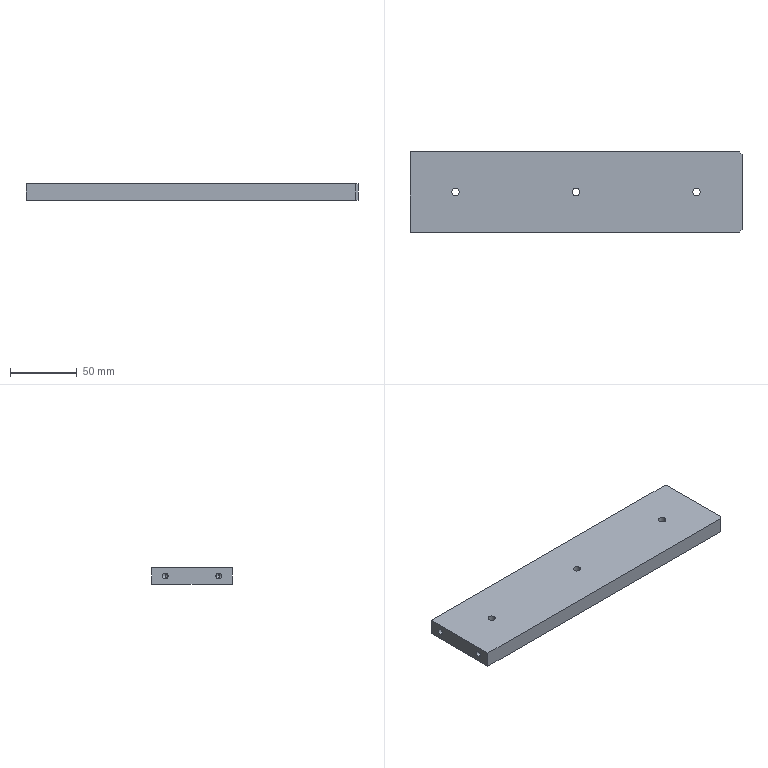Part | SolidWorks | features HoleWzd 2, Chamfer 1, Extrusion 1 | 1 solid | 31 faces | box 248 x 60 x 12 mm | volume 176365 mm3 | cylinder 16 | plane 11 | cone 4 | commonest cylinder face diameters 5.5 x6 10 x6 4.2 x4
STEP:
#1=CARTESIAN_POINT('',(95.,0.,-0.3));
#2=VERTEX_POINT('',#1);
#3=CARTESIAN_POINT('',(85.,0.,-0.3));
#4=VERTEX_POINT('',#3);
#5=CARTESIAN_POINT('',(90.,0.,-0.3));
#6=DIRECTION('',(0.,0.,-1.));
#7=DIRECTION('',(-1.,0.,0.));
#8=AXIS2_PLACEMENT_3D('',#5,#6,#7);
#9=CIRCLE('',#8,5.);
#10=EDGE_CURVE('',#2,#4,#9,.T.);
#11=ORIENTED_EDGE('',*,*,#10,.F.);
#12=CARTESIAN_POINT('',(95.,0.,-6.));
#13=VERTEX_POINT('',#12);
#14=CARTESIAN_POINT('',(95.,0.,-6.));
#15=DIRECTION('',(0.,0.,-1.));
#16=VECTOR('',#15,1000.);
#17=LINE('',#14,#16);
#18=EDGE_CURVE('',#2,#13,#17,.T.);
#19=ORIENTED_EDGE('',*,*,#18,.T.);
#20=CARTESIAN_POINT('',(85.,0.,-6.));
#21=VERTEX_POINT('',#20);
#22=CARTESIAN_POINT('',(90.,0.,-6.));
#23=DIRECTION('',(0.,0.,-1.));
#24=DIRECTION('',(-1.,0.,0.));
#25=AXIS2_PLACEMENT_3D('',#22,#23,#24);
#26=CIRCLE('',#25,5.);
#27=EDGE_CURVE('',#13,#21,#26,.T.);
#28=ORIENTED_EDGE('',*,*,#27,.T.);
#29=CARTESIAN_POINT('',(85.,0.,-6.));
#30=DIRECTION('',(0.,0.,-1.));
#31=VECTOR('',#30,1000.);
#32=LINE('',#29,#31);
#33=EDGE_CURVE('',#4,#21,#32,.T.);
#34=ORIENTED_EDGE('',*,*,#33,.F.);
#35=EDGE_LOOP('',(#11,#19,#28,#34));
#36=FACE_OUTER_BOUND('',#35,.T.);
#37=CARTESIAN_POINT('',(90.,0.,-6.));
#38=DIRECTION('',(0.,0.,-1.));
#39=DIRECTION('',(-1.,0.,0.));
#40=AXIS2_PLACEMENT_3D('',#37,#38,#39);
#41=CYLINDRICAL_SURFACE('',#40,5.);
#42=ADVANCED_FACE('',(#36),#41,.F.);
#43=CARTESIAN_POINT('',(92.75,0.,6.));
#44=VERTEX_POINT('',#43);
#45=CARTESIAN_POINT('',(87.25,0.,6.));
#46=VERTEX_POINT('',#45);
#47=CARTESIAN_POINT('',(90.,0.,6.));
#48=DIRECTION('',(0.,0.,-1.));
#49=DIRECTION('',(-1.,0.,0.));
#50=AXIS2_PLACEMENT_3D('',#47,#48,#49);
#51=CIRCLE('',#50,2.75);
#52=EDGE_CURVE('',#44,#46,#51,.T.);
#53=ORIENTED_EDGE('',*,*,#52,.F.);
#54=CARTESIAN_POINT('',(92.75,0.,-0.3));
#55=VERTEX_POINT('',#54);
#56=CARTESIAN_POINT('',(92.75,0.,-6.));
#57=DIRECTION('',(0.,0.,-1.));
#58=VECTOR('',#57,1000.);
#59=LINE('',#56,#58);
#60=EDGE_CURVE('',#44,#55,#59,.T.);
#61=ORIENTED_EDGE('',*,*,#60,.T.);
#62=CARTESIAN_POINT('',(87.25,0.,-0.3));
#63=VERTEX_POINT('',#62);
#64=CARTESIAN_POINT('',(90.,0.,-0.3));
#65=DIRECTION('',(0.,0.,-1.));
#66=DIRECTION('',(-1.,0.,0.));
#67=AXIS2_PLACEMENT_3D('',#64,#65,#66);
#68=CIRCLE('',#67,2.75);
#69=EDGE_CURVE('',#55,#63,#68,.T.);
#70=ORIENTED_EDGE('',*,*,#69,.T.);
#71=CARTESIAN_POINT('',(87.25,0.,-6.));
#72=DIRECTION('',(0.,0.,-1.));
#73=VECTOR('',#72,1000.);
#74=LINE('',#71,#73);
#75=EDGE_CURVE('',#46,#63,#74,.T.);
#76=ORIENTED_EDGE('',*,*,#75,.F.);
#77=EDGE_LOOP('',(#53,#61,#70,#76));
#78=FACE_OUTER_BOUND('',#77,.T.);
#79=CARTESIAN_POINT('',(90.,0.,-6.));
#80=DIRECTION('',(0.,0.,-1.));
#81=DIRECTION('',(-1.,0.,0.));
#82=AXIS2_PLACEMENT_3D('',#79,#80,#81);
#83=CYLINDRICAL_SURFACE('',#82,2.75);
#84=ADVANCED_FACE('',(#78),#83,.F.);
#85=CARTESIAN_POINT('',(5.,0.,-0.3));
#86=VERTEX_POINT('',#85);
#87=CARTESIAN_POINT('',(-5.,0.,-0.3));
#88=VERTEX_POINT('',#87);
#89=CARTESIAN_POINT('',(0.,0.,-0.3));
#90=DIRECTION('',(0.,0.,-1.));
#91=DIRECTION('',(-1.,0.,0.));
#92=AXIS2_PLACEMENT_3D('',#89,#90,#91);
#93=CIRCLE('',#92,5.);
#94=EDGE_CURVE('',#86,#88,#93,.T.);
#95=ORIENTED_EDGE('',*,*,#94,.F.);
#96=CARTESIAN_POINT('',(5.,0.,-6.));
#97=VERTEX_POINT('',#96);
#98=CARTESIAN_POINT('',(5.,0.,-6.));
#99=DIRECTION('',(0.,0.,-1.));
#100=VECTOR('',#99,1000.);
#101=LINE('',#98,#100);
#102=EDGE_CURVE('',#86,#97,#101,.T.);
#103=ORIENTED_EDGE('',*,*,#102,.T.);
#104=CARTESIAN_POINT('',(-5.,0.,-6.));
#105=VERTEX_POINT('',#104);
#106=CARTESIAN_POINT('',(0.,0.,-6.));
#107=DIRECTION('',(0.,0.,-1.));
#108=DIRECTION('',(-1.,0.,0.));
#109=AXIS2_PLACEMENT_3D('',#106,#107,#108);
#110=CIRCLE('',#109,5.);
#111=EDGE_CURVE('',#97,#105,#110,.T.);
#112=ORIENTED_EDGE('',*,*,#111,.T.);
#113=CARTESIAN_POINT('',(-5.,0.,-6.));
#114=DIRECTION('',(0.,0.,-1.));
#115=VECTOR('',#114,1000.);
#116=LINE('',#113,#115);
#117=EDGE_CURVE('',#88,#105,#116,.T.);
#118=ORIENTED_EDGE('',*,*,#117,.F.);
#119=EDGE_LOOP('',(#95,#103,#112,#118));
#120=FACE_OUTER_BOUND('',#119,.T.);
#121=CARTESIAN_POINT('',(0.,0.,-6.));
#122=DIRECTION('',(0.,0.,-1.));
#123=DIRECTION('',(-1.,0.,0.));
#124=AXIS2_PLACEMENT_3D('',#121,#122,#123);
#125=CYLINDRICAL_SURFACE('',#124,5.);
#126=ADVANCED_FACE('',(#120),#125,.F.);
#127=CARTESIAN_POINT('',(2.75,0.,6.));
#128=VERTEX_POINT('',#127);
#129=CARTESIAN_POINT('',(-2.75,0.,6.));
#130=VERTEX_POINT('',#129);
#131=CARTESIAN_POINT('',(0.,0.,6.));
#132=DIRECTION('',(0.,0.,-1.));
#133=DIRECTION('',(-1.,0.,0.));
#134=AXIS2_PLACEMENT_3D('',#131,#132,#133);
#135=CIRCLE('',#134,2.75);
#136=EDGE_CURVE('',#128,#130,#135,.T.);
#137=ORIENTED_EDGE('',*,*,#136,.F.);
#138=CARTESIAN_POINT('',(2.75,0.,-0.3));
#139=VERTEX_POINT('',#138);
#140=CARTESIAN_POINT('',(2.75,0.,-6.));
#141=DIRECTION('',(0.,0.,-1.));
#142=VECTOR('',#141,1000.);
#143=LINE('',#140,#142);
#144=EDGE_CURVE('',#128,#139,#143,.T.);
#145=ORIENTED_EDGE('',*,*,#144,.T.);
#146=CARTESIAN_POINT('',(-2.75,0.,-0.3));
#147=VERTEX_POINT('',#146);
#148=CARTESIAN_POINT('',(0.,0.,-0.3));
#149=DIRECTION('',(0.,0.,-1.));
#150=DIRECTION('',(-1.,0.,0.));
#151=AXIS2_PLACEMENT_3D('',#148,#149,#150);
#152=CIRCLE('',#151,2.75);
#153=EDGE_CURVE('',#139,#147,#152,.T.);
#154=ORIENTED_EDGE('',*,*,#153,.T.);
#155=CARTESIAN_POINT('',(-2.75,0.,-6.));
#156=DIRECTION('',(0.,0.,-1.));
#157=VECTOR('',#156,1000.);
#158=LINE('',#155,#157);
#159=EDGE_CURVE('',#130,#147,#158,.T.);
#160=ORIENTED_EDGE('',*,*,#159,.F.);
#161=EDGE_LOOP('',(#137,#145,#154,#160));
#162=FACE_OUTER_BOUND('',#161,.T.);
#163=CARTESIAN_POINT('',(0.,0.,-6.));
#164=DIRECTION('',(0.,0.,-1.));
#165=DIRECTION('',(-1.,0.,0.));
#166=AXIS2_PLACEMENT_3D('',#163,#164,#165);
#167=CYLINDRICAL_SURFACE('',#166,2.75);
#168=ADVANCED_FACE('',(#162),#167,.F.);
#169=CARTESIAN_POINT('',(-85.,0.,-0.3));
#170=VERTEX_POINT('',#169);
#171=CARTESIAN_POINT('',(-95.,0.,-0.3));
#172=VERTEX_POINT('',#171);
#173=CARTESIAN_POINT('',(-90.,0.,-0.3));
#174=DIRECTION('',(0.,0.,-1.));
#175=DIRECTION('',(-1.,0.,0.));
#176=AXIS2_PLACEMENT_3D('',#173,#174,#175);
#177=CIRCLE('',#176,5.);
#178=EDGE_CURVE('',#170,#172,#177,.T.);
#179=ORIENTED_EDGE('',*,*,#178,.F.);
#180=CARTESIAN_POINT('',(-85.,0.,-6.));
#181=VERTEX_POINT('',#180);
#182=CARTESIAN_POINT('',(-85.,0.,-6.));
#183=DIRECTION('',(0.,0.,-1.));
#184=VECTOR('',#183,1000.);
#185=LINE('',#182,#184);
#186=EDGE_CURVE('',#170,#181,#185,.T.);
#187=ORIENTED_EDGE('',*,*,#186,.T.);
#188=CARTESIAN_POINT('',(-95.,0.,-6.));
#189=VERTEX_POINT('',#188);
#190=CARTESIAN_POINT('',(-90.,0.,-6.));
#191=DIRECTION('',(0.,0.,-1.));
#192=DIRECTION('',(-1.,0.,0.));
#193=AXIS2_PLACEMENT_3D('',#190,#191,#192);
#194=CIRCLE('',#193,5.);
#195=EDGE_CURVE('',#181,#189,#194,.T.);
#196=ORIENTED_EDGE('',*,*,#195,.T.);
#197=CARTESIAN_POINT('',(-95.,0.,-6.));
#198=DIRECTION('',(0.,0.,-1.));
#199=VECTOR('',#198,1000.);
#200=LINE('',#197,#199);
#201=EDGE_CURVE('',#172,#189,#200,.T.);
#202=ORIENTED_EDGE('',*,*,#201,.F.);
#203=EDGE_LOOP('',(#179,#187,#196,#202));
#204=FACE_OUTER_BOUND('',#203,.T.);
#205=CARTESIAN_POINT('',(-90.,0.,-6.));
#206=DIRECTION('',(0.,0.,-1.));
#207=DIRECTION('',(-1.,0.,0.));
#208=AXIS2_PLACEMENT_3D('',#205,#206,#207);
#209=CYLINDRICAL_SURFACE('',#208,5.);
#210=ADVANCED_FACE('',(#204),#209,.F.);
#211=CARTESIAN_POINT('',(-87.25,0.,6.));
#212=VERTEX_POINT('',#211);
#213=CARTESIAN_POINT('',(-92.75,0.,6.));
#214=VERTEX_POINT('',#213);
#215=CARTESIAN_POINT('',(-90.,0.,6.));
#216=DIRECTION('',(0.,0.,-1.));
#217=DIRECTION('',(-1.,0.,0.));
#218=AXIS2_PLACEMENT_3D('',#215,#216,#217);
#219=CIRCLE('',#218,2.75);
#220=EDGE_CURVE('',#212,#214,#219,.T.);
#221=ORIENTED_EDGE('',*,*,#220,.F.);
#222=CARTESIAN_POINT('',(-87.25,0.,-0.3));
#223=VERTEX_POINT('',#222);
#224=CARTESIAN_POINT('',(-87.25,0.,-6.));
#225=DIRECTION('',(0.,0.,-1.));
#226=VECTOR('',#225,1000.);
#227=LINE('',#224,#226);
#228=EDGE_CURVE('',#212,#223,#227,.T.);
#229=ORIENTED_EDGE('',*,*,#228,.T.);
#230=CARTESIAN_POINT('',(-92.75,0.,-0.3));
#231=VERTEX_POINT('',#230);
#232=CARTESIAN_POINT('',(-90.,0.,-0.3));
#233=DIRECTION('',(0.,0.,-1.));
#234=DIRECTION('',(-1.,0.,0.));
#235=AXIS2_PLACEMENT_3D('',#232,#233,#234);
#236=CIRCLE('',#235,2.75);
#237=EDGE_CURVE('',#223,#231,#236,.T.);
#238=ORIENTED_EDGE('',*,*,#237,.T.);
#239=CARTESIAN_POINT('',(-92.75,0.,-6.));
#240=DIRECTION('',(0.,0.,-1.));
#241=VECTOR('',#240,1000.);
#242=LINE('',#239,#241);
#243=EDGE_CURVE('',#214,#231,#242,.T.);
#244=ORIENTED_EDGE('',*,*,#243,.F.);
#245=EDGE_LOOP('',(#221,#229,#238,#244));
#246=FACE_OUTER_BOUND('',#245,.T.);
#247=CARTESIAN_POINT('',(-90.,0.,-6.));
#248=DIRECTION('',(0.,0.,-1.));
#249=DIRECTION('',(-1.,0.,0.));
#250=AXIS2_PLACEMENT_3D('',#247,#248,#249);
#251=CYLINDRICAL_SURFACE('',#250,2.75);
#252=ADVANCED_FACE('',(#246),#251,.F.);
#253=CARTESIAN_POINT('',(-111.6,20.,-2.1));
#254=VERTEX_POINT('',#253);
#255=CARTESIAN_POINT('',(-111.6,20.,2.1));
#256=VERTEX_POINT('',#255);
#257=CARTESIAN_POINT('',(-111.6,20.,0.));
#258=DIRECTION('',(-1.,0.,0.));
#259=DIRECTION('',(0.,0.,1.));
#260=AXIS2_PLACEMENT_3D('',#257,#258,#259);
#261=CIRCLE('',#260,2.1);
#262=EDGE_CURVE('',#254,#256,#261,.T.);
#263=ORIENTED_EDGE('',*,*,#262,.F.);
#264=CARTESIAN_POINT('',(-124.,20.,-2.1));
#265=VERTEX_POINT('',#264);
#266=CARTESIAN_POINT('',(-124.,20.,-2.1));
#267=DIRECTION('',(-1.,0.,0.));
#268=VECTOR('',#267,1000.);
#269=LINE('',#266,#268);
#270=EDGE_CURVE('',#254,#265,#269,.T.);
#271=ORIENTED_EDGE('',*,*,#270,.T.);
#272=CARTESIAN_POINT('',(-124.,20.,2.1));
#273=VERTEX_POINT('',#272);
#274=CARTESIAN_POINT('',(-124.,20.,0.));
#275=DIRECTION('',(-1.,0.,0.));
#276=DIRECTION('',(0.,0.,1.));
#277=AXIS2_PLACEMENT_3D('',#274,#275,#276);
#278=CIRCLE('',#277,2.1);
#279=EDGE_CURVE('',#265,#273,#278,.T.);
#280=ORIENTED_EDGE('',*,*,#279,.T.);
#281=CARTESIAN_POINT('',(-124.,20.,2.1));
#282=DIRECTION('',(-1.,0.,0.));
#283=VECTOR('',#282,1000.);
#284=LINE('',#281,#283);
#285=EDGE_CURVE('',#256,#273,#284,.T.);
#286=ORIENTED_EDGE('',*,*,#285,.F.);
#287=EDGE_LOOP('',(#263,#271,#280,#286));
#288=FACE_OUTER_BOUND('',#287,.T.);
#289=CARTESIAN_POINT('',(-124.,20.,0.));
#290=DIRECTION('',(-1.,0.,0.));
#291=DIRECTION('',(0.,0.,1.));
#292=AXIS2_PLACEMENT_3D('',#289,#290,#291);
#293=CYLINDRICAL_SURFACE('',#292,2.1);
#294=ADVANCED_FACE('',(#288),#293,.F.);
#295=CARTESIAN_POINT('',(-110.338,20.,0.));
#296=VERTEX_POINT('',#295);
#297=CARTESIAN_POINT('',(-111.6,20.,2.1));
#298=DIRECTION('',(-0.515,0.,0.8572));
#299=VECTOR('',#298,1000.);
#300=LINE('',#297,#299);
#301=EDGE_CURVE('',#296,#256,#300,.T.);
#302=ORIENTED_EDGE('',*,*,#301,.F.);
#303=CARTESIAN_POINT('',(-111.6,20.,-2.1));
#304=DIRECTION('',(-0.515,0.,-0.8572));
#305=VECTOR('',#304,1000.);
#306=LINE('',#303,#305);
#307=EDGE_CURVE('',#296,#254,#306,.T.);
#308=ORIENTED_EDGE('',*,*,#307,.T.);
#309=ORIENTED_EDGE('',*,*,#262,.T.);
#310=EDGE_LOOP('',(#302,#308,#309));
#311=FACE_OUTER_BOUND('',#310,.T.);
#312=CARTESIAN_POINT('',(-111.6,20.,0.));
#313=DIRECTION('',(-1.,0.,0.));
#314=DIRECTION('',(0.,0.,1.));
#315=AXIS2_PLACEMENT_3D('',#312,#313,#314);
#316=CONICAL_SURFACE('',#315,2.1,1.03);
#317=ADVANCED_FACE('',(#311),#316,.F.);
#318=CARTESIAN_POINT('',(-111.6,-20.,-2.1));
#319=VERTEX_POINT('',#318);
#320=CARTESIAN_POINT('',(-111.6,-20.,2.1));
#321=VERTEX_POINT('',#320);
#322=CARTESIAN_POINT('',(-111.6,-20.,0.));
#323=DIRECTION('',(-1.,0.,0.));
#324=DIRECTION('',(0.,0.,1.));
#325=AXIS2_PLACEMENT_3D('',#322,#323,#324);
#326=CIRCLE('',#325,2.1);
#327=EDGE_CURVE('',#319,#321,#326,.T.);
#328=ORIENTED_EDGE('',*,*,#327,.F.);
#329=CARTESIAN_POINT('',(-124.,-20.,-2.1));
#330=VERTEX_POINT('',#329);
#331=CARTESIAN_POINT('',(-124.,-20.,-2.1));
#332=DIRECTION('',(-1.,0.,0.));
#333=VECTOR('',#332,1000.);
#334=LINE('',#331,#333);
#335=EDGE_CURVE('',#319,#330,#334,.T.);
#336=ORIENTED_EDGE('',*,*,#335,.T.);
#337=CARTESIAN_POINT('',(-124.,-20.,2.1));
#338=VERTEX_POINT('',#337);
#339=CARTESIAN_POINT('',(-124.,-20.,0.));
#340=DIRECTION('',(-1.,0.,0.));
#341=DIRECTION('',(0.,0.,1.));
#342=AXIS2_PLACEMENT_3D('',#339,#340,#341);
#343=CIRCLE('',#342,2.1);
#344=EDGE_CURVE('',#330,#338,#343,.T.);
#345=ORIENTED_EDGE('',*,*,#344,.T.);
#346=CARTESIAN_POINT('',(-124.,-20.,2.1));
#347=DIRECTION('',(-1.,0.,0.));
#348=VECTOR('',#347,1000.);
#349=LINE('',#346,#348);
#350=EDGE_CURVE('',#321,#338,#349,.T.);
#351=ORIENTED_EDGE('',*,*,#350,.F.);
#352=EDGE_LOOP('',(#328,#336,#345,#351));
#353=FACE_OUTER_BOUND('',#352,.T.);
#354=CARTESIAN_POINT('',(-124.,-20.,0.));
#355=DIRECTION('',(-1.,0.,0.));
#356=DIRECTION('',(0.,0.,1.));
#357=AXIS2_PLACEMENT_3D('',#354,#355,#356);
#358=CYLINDRICAL_SURFACE('',#357,2.1);
#359=ADVANCED_FACE('',(#353),#358,.F.);
#360=CARTESIAN_POINT('',(-110.338,-20.,0.));
#361=VERTEX_POINT('',#360);
#362=CARTESIAN_POINT('',(-111.6,-20.,2.1));
#363=DIRECTION('',(-0.515,0.,0.8572));
#364=VECTOR('',#363,1000.);
#365=LINE('',#362,#364);
#366=EDGE_CURVE('',#361,#321,#365,.T.);
#367=ORIENTED_EDGE('',*,*,#366,.F.);
#368=CARTESIAN_POINT('',(-111.6,-20.,-2.1));
#369=DIRECTION('',(-0.515,0.,-0.8572));
#370=VECTOR('',#369,1000.);
#371=LINE('',#368,#370);
#372=EDGE_CURVE('',#361,#319,#371,.T.);
#373=ORIENTED_EDGE('',*,*,#372,.T.);
#374=ORIENTED_EDGE('',*,*,#327,.T.);
#375=EDGE_LOOP('',(#367,#373,#374));
#376=FACE_OUTER_BOUND('',#375,.T.);
#377=CARTESIAN_POINT('',(-111.6,-20.,0.));
#378=DIRECTION('',(-1.,0.,0.));
#379=DIRECTION('',(0.,0.,1.));
#380=AXIS2_PLACEMENT_3D('',#377,#378,#379);
#381=CONICAL_SURFACE('',#380,2.1,1.03);
#382=ADVANCED_FACE('',(#376),#381,.F.);
#383=CARTESIAN_POINT('',(124.,-28.,6.));
#384=VERTEX_POINT('',#383);
#385=CARTESIAN_POINT('',(124.,28.,6.));
#386=VERTEX_POINT('',#385);
#387=CARTESIAN_POINT('',(124.,-30.,6.));
#388=DIRECTION('',(0.,1.,0.));
#389=VECTOR('',#388,1000.);
#390=LINE('',#387,#389);
#391=EDGE_CURVE('',#384,#386,#390,.T.);
#392=ORIENTED_EDGE('',*,*,#391,.F.);
#393=CARTESIAN_POINT('',(124.,-28.,-6.));
#394=VERTEX_POINT('',#393);
#395=CARTESIAN_POINT('',(124.,-28.,6.));
#396=DIRECTION('',(0.,0.,-1.));
#397=VECTOR('',#396,1000.);
#398=LINE('',#395,#397);
#399=EDGE_CURVE('',#384,#394,#398,.T.);
#400=ORIENTED_EDGE('',*,*,#399,.T.);
#401=CARTESIAN_POINT('',(124.,28.,-6.));
#402=VERTEX_POINT('',#401);
#403=CARTESIAN_POINT('',(124.,-30.,-6.));
#404=DIRECTION('',(0.,1.,0.));
#405=VECTOR('',#404,1000.);
#406=LINE('',#403,#405);
#407=EDGE_CURVE('',#394,#402,#406,.T.);
#408=ORIENTED_EDGE('',*,*,#407,.T.);
#409=CARTESIAN_POINT('',(124.,28.,6.));
#410=DIRECTION('',(0.,0.,1.));
#411=VECTOR('',#410,1000.);
#412=LINE('',#409,#411);
#413=EDGE_CURVE('',#402,#386,#412,.T.);
#414=ORIENTED_EDGE('',*,*,#413,.T.);
#415=EDGE_LOOP('',(#392,#400,#408,#414));
#416=FACE_OUTER_BOUND('',#415,.T.);
#417=CARTESIAN_POINT('',(124.,-30.,6.));
#418=DIRECTION('',(-1.,0.,0.));
#419=DIRECTION('',(0.,0.,1.));
#420=AXIS2_PLACEMENT_3D('',#417,#418,#419);
#421=PLANE('',#420);
#422=ADVANCED_FACE('',(#416),#421,.F.);
#423=CARTESIAN_POINT('',(122.,30.,6.));
#424=VERTEX_POINT('',#423);
#425=CARTESIAN_POINT('',(-124.,30.,6.));
#426=VERTEX_POINT('',#425);
#427=CARTESIAN_POINT('',(-124.,30.,6.));
#428=DIRECTION('',(-1.,0.,0.));
#429=VECTOR('',#428,1000.);
#430=LINE('',#427,#429);
#431=EDGE_CURVE('',#424,#426,#430,.T.);
#432=ORIENTED_EDGE('',*,*,#431,.F.);
#433=CARTESIAN_POINT('',(122.,30.,-6.));
#434=VERTEX_POINT('',#433);
#435=CARTESIAN_POINT('',(122.,30.,6.));
#436=DIRECTION('',(0.,0.,-1.));
#437=VECTOR('',#436,1000.);
#438=LINE('',#435,#437);
#439=EDGE_CURVE('',#424,#434,#438,.T.);
#440=ORIENTED_EDGE('',*,*,#439,.T.);
#441=CARTESIAN_POINT('',(-124.,30.,-6.));
#442=VERTEX_POINT('',#441);
#443=CARTESIAN_POINT('',(-124.,30.,-6.));
#444=DIRECTION('',(-1.,0.,0.));
#445=VECTOR('',#444,1000.);
#446=LINE('',#443,#445);
#447=EDGE_CURVE('',#434,#442,#446,.T.);
#448=ORIENTED_EDGE('',*,*,#447,.T.);
#449=CARTESIAN_POINT('',(-124.,30.,6.));
#450=DIRECTION('',(0.,0.,-1.));
#451=VECTOR('',#450,1000.);
#452=LINE('',#449,#451);
#453=EDGE_CURVE('',#426,#442,#452,.T.);
#454=ORIENTED_EDGE('',*,*,#453,.F.);
#455=EDGE_LOOP('',(#432,#440,#448,#454));
#456=FACE_OUTER_BOUND('',#455,.T.);
#457=CARTESIAN_POINT('',(-124.,30.,6.));
#458=DIRECTION('',(0.,-1.,0.));
#459=DIRECTION('',(0.,0.,-1.));
#460=AXIS2_PLACEMENT_3D('',#457,#458,#459);
#461=PLANE('',#460);
#462=ADVANCED_FACE('',(#456),#461,.F.);
#463=CARTESIAN_POINT('',(-124.,20.,0.));
#464=DIRECTION('',(-1.,0.,0.));
#465=DIRECTION('',(0.,0.,1.));
#466=AXIS2_PLACEMENT_3D('',#463,#464,#465);
#467=CIRCLE('',#466,2.1);
#468=EDGE_CURVE('',#273,#265,#467,.T.);
#469=ORIENTED_EDGE('',*,*,#468,.F.);
#470=ORIENTED_EDGE('',*,*,#279,.F.);
#471=EDGE_LOOP('',(#469,#470));
#472=FACE_BOUND('',#471,.T.);
#473=CARTESIAN_POINT('',(-124.,-20.,0.));
#474=DIRECTION('',(-1.,0.,0.));
#475=DIRECTION('',(0.,0.,1.));
#476=AXIS2_PLACEMENT_3D('',#473,#474,#475);
#477=CIRCLE('',#476,2.1);
#478=EDGE_CURVE('',#338,#330,#477,.T.);
#479=ORIENTED_EDGE('',*,*,#478,.F.);
#480=ORIENTED_EDGE('',*,*,#344,.F.);
#481=EDGE_LOOP('',(#479,#480));
#482=FACE_BOUND('',#481,.T.);
#483=CARTESIAN_POINT('',(-124.,-30.,-6.));
#484=VERTEX_POINT('',#483);
#485=CARTESIAN_POINT('',(-124.,-30.,-6.));
#486=DIRECTION('',(0.,-1.,0.));
#487=VECTOR('',#486,1000.);
#488=LINE('',#485,#487);
#489=EDGE_CURVE('',#442,#484,#488,.T.);
#490=ORIENTED_EDGE('',*,*,#489,.T.);
#491=CARTESIAN_POINT('',(-124.,-30.,6.));
#492=VERTEX_POINT('',#491);
#493=CARTESIAN_POINT('',(-124.,-30.,6.));
#494=DIRECTION('',(0.,0.,-1.));
#495=VECTOR('',#494,1000.);
#496=LINE('',#493,#495);
#497=EDGE_CURVE('',#492,#484,#496,.T.);
#498=ORIENTED_EDGE('',*,*,#497,.F.);
#499=CARTESIAN_POINT('',(-124.,-30.,6.));
#500=DIRECTION('',(0.,-1.,0.));
#501=VECTOR('',#500,1000.);
#502=LINE('',#499,#501);
#503=EDGE_CURVE('',#426,#492,#502,.T.);
#504=ORIENTED_EDGE('',*,*,#503,.F.);
#505=ORIENTED_EDGE('',*,*,#453,.T.);
#506=EDGE_LOOP('',(#490,#498,#504,#505));
#507=FACE_OUTER_BOUND('',#506,.T.);
#508=CARTESIAN_POINT('',(-124.,-30.,6.));
#509=DIRECTION('',(1.,0.,0.));
#510=DIRECTION('',(0.,0.,-1.));
#511=AXIS2_PLACEMENT_3D('',#508,#509,#510);
#512=PLANE('',#511);
#513=ADVANCED_FACE('',(#472,#482,#507),#512,.F.);
#514=CARTESIAN_POINT('',(122.,-30.,-6.));
#515=VERTEX_POINT('',#514);
#516=CARTESIAN_POINT('',(-124.,-30.,-6.));
#517=DIRECTION('',(1.,0.,0.));
#518=VECTOR('',#517,1000.);
#519=LINE('',#516,#518);
#520=EDGE_CURVE('',#484,#515,#519,.T.);
#521=ORIENTED_EDGE('',*,*,#520,.T.);
#522=CARTESIAN_POINT('',(122.,-30.,6.));
#523=VERTEX_POINT('',#522);
#524=CARTESIAN_POINT('',(122.,-30.,6.));
#525=DIRECTION('',(0.,0.,1.));
#526=VECTOR('',#525,1000.);
#527=LINE('',#524,#526);
#528=EDGE_CURVE('',#515,#523,#527,.T.);
#529=ORIENTED_EDGE('',*,*,#528,.T.);
#530=CARTESIAN_POINT('',(-124.,-30.,6.));
#531=DIRECTION('',(1.,0.,0.));
#532=VECTOR('',#531,1000.);
#533=LINE('',#530,#532);
#534=EDGE_CURVE('',#492,#523,#533,.T.);
#535=ORIENTED_EDGE('',*,*,#534,.F.);
#536=ORIENTED_EDGE('',*,*,#497,.T.);
#537=EDGE_LOOP('',(#521,#529,#535,#536));
#538=FACE_OUTER_BOUND('',#537,.T.);
#539=CARTESIAN_POINT('',(-124.,-30.,6.));
#540=DIRECTION('',(0.,1.,0.));
#541=DIRECTION('',(0.,0.,1.));
#542=AXIS2_PLACEMENT_3D('',#539,#540,#541);
#543=PLANE('',#542);
#544=ADVANCED_FACE('',(#538),#543,.F.);
#545=CARTESIAN_POINT('',(90.,0.,6.));
#546=DIRECTION('',(0.,0.,-1.));
#547=DIRECTION('',(-1.,0.,0.));
#548=AXIS2_PLACEMENT_3D('',#545,#546,#547);
#549=CIRCLE('',#548,2.75);
#550=EDGE_CURVE('',#46,#44,#549,.T.);
#551=ORIENTED_EDGE('',*,*,#550,.T.);
#552=ORIENTED_EDGE('',*,*,#52,.T.);
#553=EDGE_LOOP('',(#551,#552));
#554=FACE_BOUND('',#553,.T.);
#555=CARTESIAN_POINT('',(0.,0.,6.));
#556=DIRECTION('',(0.,0.,-1.));
#557=DIRECTION('',(-1.,0.,0.));
#558=AXIS2_PLACEMENT_3D('',#555,#556,#557);
#559=CIRCLE('',#558,2.75);
#560=EDGE_CURVE('',#130,#128,#559,.T.);
#561=ORIENTED_EDGE('',*,*,#560,.T.);
#562=ORIENTED_EDGE('',*,*,#136,.T.);
#563=EDGE_LOOP('',(#561,#562));
#564=FACE_BOUND('',#563,.T.);
#565=CARTESIAN_POINT('',(-90.,0.,6.));
#566=DIRECTION('',(0.,0.,-1.));
#567=DIRECTION('',(-1.,0.,0.));
#568=AXIS2_PLACEMENT_3D('',#565,#566,#567);
#569=CIRCLE('',#568,2.75);
#570=EDGE_CURVE('',#214,#212,#569,.T.);
#571=ORIENTED_EDGE('',*,*,#570,.T.);
#572=ORIENTED_EDGE('',*,*,#220,.T.);
#573=EDGE_LOOP('',(#571,#572));
#574=FACE_BOUND('',#573,.T.);
#575=ORIENTED_EDGE('',*,*,#534,.T.);
#576=CARTESIAN_POINT('',(124.,-28.,6.));
#577=DIRECTION('',(0.7071,0.7071,0.));
#578=VECTOR('',#577,1000.);
#579=LINE('',#576,#578);
#580=EDGE_CURVE('',#523,#384,#579,.T.);
#581=ORIENTED_EDGE('',*,*,#580,.T.);
#582=ORIENTED_EDGE('',*,*,#391,.T.);
#583=CARTESIAN_POINT('',(122.,30.,6.));
#584=DIRECTION('',(-0.7071,0.7071,0.));
#585=VECTOR('',#584,1000.);
#586=LINE('',#583,#585);
#587=EDGE_CURVE('',#386,#424,#586,.T.);
#588=ORIENTED_EDGE('',*,*,#587,.T.);
#589=ORIENTED_EDGE('',*,*,#431,.T.);
#590=ORIENTED_EDGE('',*,*,#503,.T.);
#591=EDGE_LOOP('',(#575,#581,#582,#588,#589,#590));
#592=FACE_OUTER_BOUND('',#591,.T.);
#593=CARTESIAN_POINT('',(0.,0.,6.));
#594=DIRECTION('',(0.,0.,-1.));
#595=DIRECTION('',(-1.,0.,0.));
#596=AXIS2_PLACEMENT_3D('',#593,#594,#595);
#597=PLANE('',#596);
#598=ADVANCED_FACE('',(#554,#564,#574,#592),#597,.F.);
#599=CARTESIAN_POINT('',(90.,0.,-6.));
#600=DIRECTION('',(0.,0.,-1.));
#601=DIRECTION('',(-1.,0.,0.));
#602=AXIS2_PLACEMENT_3D('',#599,#600,#601);
#603=CIRCLE('',#602,5.);
#604=EDGE_CURVE('',#21,#13,#603,.T.);
#605=ORIENTED_EDGE('',*,*,#604,.F.);
#606=ORIENTED_EDGE('',*,*,#27,.F.);
#607=EDGE_LOOP('',(#605,#606));
#608=FACE_BOUND('',#607,.T.);
#609=CARTESIAN_POINT('',(0.,0.,-6.));
#610=DIRECTION('',(0.,0.,-1.));
#611=DIRECTION('',(-1.,0.,0.));
#612=AXIS2_PLACEMENT_3D('',#609,#610,#611);
#613=CIRCLE('',#612,5.);
#614=EDGE_CURVE('',#105,#97,#613,.T.);
#615=ORIENTED_EDGE('',*,*,#614,.F.);
#616=ORIENTED_EDGE('',*,*,#111,.F.);
#617=EDGE_LOOP('',(#615,#616));
#618=FACE_BOUND('',#617,.T.);
#619=CARTESIAN_POINT('',(-90.,0.,-6.));
#620=DIRECTION('',(0.,0.,-1.));
#621=DIRECTION('',(-1.,0.,0.));
#622=AXIS2_PLACEMENT_3D('',#619,#620,#621);
#623=CIRCLE('',#622,5.);
#624=EDGE_CURVE('',#189,#181,#623,.T.);
#625=ORIENTED_EDGE('',*,*,#624,.F.);
#626=ORIENTED_EDGE('',*,*,#195,.F.);
#627=EDGE_LOOP('',(#625,#626));
#628=FACE_BOUND('',#627,.T.);
#629=ORIENTED_EDGE('',*,*,#407,.F.);
#630=CARTESIAN_POINT('',(76.,-76.,-6.));
#631=DIRECTION('',(-0.7071,-0.7071,0.));
#632=VECTOR('',#631,1000.);
#633=LINE('',#630,#632);
#634=EDGE_CURVE('',#394,#515,#633,.T.);
#635=ORIENTED_EDGE('',*,*,#634,.T.);
#636=ORIENTED_EDGE('',*,*,#520,.F.);
#637=ORIENTED_EDGE('',*,*,#489,.F.);
#638=ORIENTED_EDGE('',*,*,#447,.F.);
#639=CARTESIAN_POINT('',(76.,76.,-6.));
#640=DIRECTION('',(0.7071,-0.7071,0.));
#641=VECTOR('',#640,1000.);
#642=LINE('',#639,#641);
#643=EDGE_CURVE('',#434,#402,#642,.T.);
#644=ORIENTED_EDGE('',*,*,#643,.T.);
#645=EDGE_LOOP('',(#629,#635,#636,#637,#638,#644));
#646=FACE_OUTER_BOUND('',#645,.T.);
#647=CARTESIAN_POINT('',(0.,0.,-6.));
#648=DIRECTION('',(0.,0.,-1.));
#649=DIRECTION('',(-1.,0.,0.));
#650=AXIS2_PLACEMENT_3D('',#647,#648,#649);
#651=PLANE('',#650);
#652=ADVANCED_FACE('',(#608,#618,#628,#646),#651,.T.);
#653=ORIENTED_EDGE('',*,*,#372,.F.);
#654=ORIENTED_EDGE('',*,*,#366,.T.);
#655=CARTESIAN_POINT('',(-111.6,-20.,0.));
#656=DIRECTION('',(-1.,0.,0.));
#657=DIRECTION('',(0.,0.,1.));
#658=AXIS2_PLACEMENT_3D('',#655,#656,#657);
#659=CIRCLE('',#658,2.1);
#660=EDGE_CURVE('',#321,#319,#659,.T.);
#661=ORIENTED_EDGE('',*,*,#660,.T.);
#662=EDGE_LOOP('',(#653,#654,#661));
#663=FACE_OUTER_BOUND('',#662,.T.);
#664=CARTESIAN_POINT('',(-111.6,-20.,0.));
#665=DIRECTION('',(-1.,0.,0.));
#666=DIRECTION('',(0.,0.,1.));
#667=AXIS2_PLACEMENT_3D('',#664,#665,#666);
#668=CONICAL_SURFACE('',#667,2.1,1.03);
#669=ADVANCED_FACE('',(#663),#668,.F.);
#670=ORIENTED_EDGE('',*,*,#335,.F.);
#671=ORIENTED_EDGE('',*,*,#660,.F.);
#672=ORIENTED_EDGE('',*,*,#350,.T.);
#673=ORIENTED_EDGE('',*,*,#478,.T.);
#674=EDGE_LOOP('',(#670,#671,#672,#673));
#675=FACE_OUTER_BOUND('',#674,.T.);
#676=CARTESIAN_POINT('',(-124.,-20.,0.));
#677=DIRECTION('',(-1.,0.,0.));
#678=DIRECTION('',(0.,0.,1.));
#679=AXIS2_PLACEMENT_3D('',#676,#677,#678);
#680=CYLINDRICAL_SURFACE('',#679,2.1);
#681=ADVANCED_FACE('',(#675),#680,.F.);
#682=ORIENTED_EDGE('',*,*,#307,.F.);
#683=ORIENTED_EDGE('',*,*,#301,.T.);
#684=CARTESIAN_POINT('',(-111.6,20.,0.));
#685=DIRECTION('',(-1.,0.,0.));
#686=DIRECTION('',(0.,0.,1.));
#687=AXIS2_PLACEMENT_3D('',#684,#685,#686);
#688=CIRCLE('',#687,2.1);
#689=EDGE_CURVE('',#256,#254,#688,.T.);
#690=ORIENTED_EDGE('',*,*,#689,.T.);
#691=EDGE_LOOP('',(#682,#683,#690));
#692=FACE_OUTER_BOUND('',#691,.T.);
#693=CARTESIAN_POINT('',(-111.6,20.,0.));
#694=DIRECTION('',(-1.,0.,0.));
#695=DIRECTION('',(0.,0.,1.));
#696=AXIS2_PLACEMENT_3D('',#693,#694,#695);
#697=CONICAL_SURFACE('',#696,2.1,1.03);
#698=ADVANCED_FACE('',(#692),#697,.F.);
#699=ORIENTED_EDGE('',*,*,#270,.F.);
#700=ORIENTED_EDGE('',*,*,#689,.F.);
#701=ORIENTED_EDGE('',*,*,#285,.T.);
#702=ORIENTED_EDGE('',*,*,#468,.T.);
#703=EDGE_LOOP('',(#699,#700,#701,#702));
#704=FACE_OUTER_BOUND('',#703,.T.);
#705=CARTESIAN_POINT('',(-124.,20.,0.));
#706=DIRECTION('',(-1.,0.,0.));
#707=DIRECTION('',(0.,0.,1.));
#708=AXIS2_PLACEMENT_3D('',#705,#706,#707);
#709=CYLINDRICAL_SURFACE('',#708,2.1);
#710=ADVANCED_FACE('',(#704),#709,.F.);
#711=ORIENTED_EDGE('',*,*,#580,.F.);
#712=ORIENTED_EDGE('',*,*,#528,.F.);
#713=ORIENTED_EDGE('',*,*,#634,.F.);
#714=ORIENTED_EDGE('',*,*,#399,.F.);
#715=EDGE_LOOP('',(#711,#712,#713,#714));
#716=FACE_OUTER_BOUND('',#715,.T.);
#717=CARTESIAN_POINT('',(124.,-28.,6.));
#718=DIRECTION('',(-0.7071,0.7071,0.));
#719=DIRECTION('',(0.,0.,-1.));
#720=AXIS2_PLACEMENT_3D('',#717,#718,#719);
#721=PLANE('',#720);
#722=ADVANCED_FACE('',(#716),#721,.F.);
#723=ORIENTED_EDGE('',*,*,#587,.F.);
#724=ORIENTED_EDGE('',*,*,#413,.F.);
#725=ORIENTED_EDGE('',*,*,#643,.F.);
#726=ORIENTED_EDGE('',*,*,#439,.F.);
#727=EDGE_LOOP('',(#723,#724,#725,#726));
#728=FACE_OUTER_BOUND('',#727,.T.);
#729=CARTESIAN_POINT('',(122.,30.,6.));
#730=DIRECTION('',(-0.7071,-0.7071,0.));
#731=DIRECTION('',(0.,0.,-1.));
#732=AXIS2_PLACEMENT_3D('',#729,#730,#731);
#733=PLANE('',#732);
#734=ADVANCED_FACE('',(#728),#733,.F.);
#735=ORIENTED_EDGE('',*,*,#228,.F.);
#736=ORIENTED_EDGE('',*,*,#570,.F.);
#737=ORIENTED_EDGE('',*,*,#243,.T.);
#738=CARTESIAN_POINT('',(-90.,0.,-0.3));
#739=DIRECTION('',(0.,0.,-1.));
#740=DIRECTION('',(-1.,0.,0.));
#741=AXIS2_PLACEMENT_3D('',#738,#739,#740);
#742=CIRCLE('',#741,2.75);
#743=EDGE_CURVE('',#231,#223,#742,.T.);
#744=ORIENTED_EDGE('',*,*,#743,.T.);
#745=EDGE_LOOP('',(#735,#736,#737,#744));
#746=FACE_OUTER_BOUND('',#745,.T.);
#747=CARTESIAN_POINT('',(-90.,0.,-6.));
#748=DIRECTION('',(0.,0.,-1.));
#749=DIRECTION('',(-1.,0.,0.));
#750=AXIS2_PLACEMENT_3D('',#747,#748,#749);
#751=CYLINDRICAL_SURFACE('',#750,2.75);
#752=ADVANCED_FACE('',(#746),#751,.F.);
#753=ORIENTED_EDGE('',*,*,#743,.F.);
#754=ORIENTED_EDGE('',*,*,#237,.F.);
#755=EDGE_LOOP('',(#753,#754));
#756=FACE_BOUND('',#755,.T.);
#757=CARTESIAN_POINT('',(-90.,0.,-0.3));
#758=DIRECTION('',(0.,0.,-1.));
#759=DIRECTION('',(-1.,0.,0.));
#760=AXIS2_PLACEMENT_3D('',#757,#758,#759);
#761=CIRCLE('',#760,5.);
#762=EDGE_CURVE('',#172,#170,#761,.T.);
#763=ORIENTED_EDGE('',*,*,#762,.T.);
#764=ORIENTED_EDGE('',*,*,#178,.T.);
#765=EDGE_LOOP('',(#763,#764));
#766=FACE_OUTER_BOUND('',#765,.T.);
#767=CARTESIAN_POINT('',(-87.25,0.,-0.3));
#768=DIRECTION('',(0.,0.,1.));
#769=DIRECTION('',(1.,0.,0.));
#770=AXIS2_PLACEMENT_3D('',#767,#768,#769);
#771=PLANE('',#770);
#772=ADVANCED_FACE('',(#756,#766),#771,.F.);
#773=ORIENTED_EDGE('',*,*,#186,.F.);
#774=ORIENTED_EDGE('',*,*,#762,.F.);
#775=ORIENTED_EDGE('',*,*,#201,.T.);
#776=ORIENTED_EDGE('',*,*,#624,.T.);
#777=EDGE_LOOP('',(#773,#774,#775,#776));
#778=FACE_OUTER_BOUND('',#777,.T.);
#779=CARTESIAN_POINT('',(-90.,0.,-6.));
#780=DIRECTION('',(0.,0.,-1.));
#781=DIRECTION('',(-1.,0.,0.));
#782=AXIS2_PLACEMENT_3D('',#779,#780,#781);
#783=CYLINDRICAL_SURFACE('',#782,5.);
#784=ADVANCED_FACE('',(#778),#783,.F.);
#785=ORIENTED_EDGE('',*,*,#144,.F.);
#786=ORIENTED_EDGE('',*,*,#560,.F.);
#787=ORIENTED_EDGE('',*,*,#159,.T.);
#788=CARTESIAN_POINT('',(0.,0.,-0.3));
#789=DIRECTION('',(0.,0.,-1.));
#790=DIRECTION('',(-1.,0.,0.));
#791=AXIS2_PLACEMENT_3D('',#788,#789,#790);
#792=CIRCLE('',#791,2.75);
#793=EDGE_CURVE('',#147,#139,#792,.T.);
#794=ORIENTED_EDGE('',*,*,#793,.T.);
#795=EDGE_LOOP('',(#785,#786,#787,#794));
#796=FACE_OUTER_BOUND('',#795,.T.);
#797=CARTESIAN_POINT('',(0.,0.,-6.));
#798=DIRECTION('',(0.,0.,-1.));
#799=DIRECTION('',(-1.,0.,0.));
#800=AXIS2_PLACEMENT_3D('',#797,#798,#799);
#801=CYLINDRICAL_SURFACE('',#800,2.75);
#802=ADVANCED_FACE('',(#796),#801,.F.);
#803=ORIENTED_EDGE('',*,*,#793,.F.);
#804=ORIENTED_EDGE('',*,*,#153,.F.);
#805=EDGE_LOOP('',(#803,#804));
#806=FACE_BOUND('',#805,.T.);
#807=CARTESIAN_POINT('',(0.,0.,-0.3));
#808=DIRECTION('',(0.,0.,-1.));
#809=DIRECTION('',(-1.,0.,0.));
#810=AXIS2_PLACEMENT_3D('',#807,#808,#809);
#811=CIRCLE('',#810,5.);
#812=EDGE_CURVE('',#88,#86,#811,.T.);
#813=ORIENTED_EDGE('',*,*,#812,.T.);
#814=ORIENTED_EDGE('',*,*,#94,.T.);
#815=EDGE_LOOP('',(#813,#814));
#816=FACE_OUTER_BOUND('',#815,.T.);
#817=CARTESIAN_POINT('',(2.75,0.,-0.3));
#818=DIRECTION('',(0.,0.,1.));
#819=DIRECTION('',(1.,0.,0.));
#820=AXIS2_PLACEMENT_3D('',#817,#818,#819);
#821=PLANE('',#820);
#822=ADVANCED_FACE('',(#806,#816),#821,.F.);
#823=ORIENTED_EDGE('',*,*,#102,.F.);
#824=ORIENTED_EDGE('',*,*,#812,.F.);
#825=ORIENTED_EDGE('',*,*,#117,.T.);
#826=ORIENTED_EDGE('',*,*,#614,.T.);
#827=EDGE_LOOP('',(#823,#824,#825,#826));
#828=FACE_OUTER_BOUND('',#827,.T.);
#829=CARTESIAN_POINT('',(0.,0.,-6.));
#830=DIRECTION('',(0.,0.,-1.));
#831=DIRECTION('',(-1.,0.,0.));
#832=AXIS2_PLACEMENT_3D('',#829,#830,#831);
#833=CYLINDRICAL_SURFACE('',#832,5.);
#834=ADVANCED_FACE('',(#828),#833,.F.);
#835=ORIENTED_EDGE('',*,*,#60,.F.);
#836=ORIENTED_EDGE('',*,*,#550,.F.);
#837=ORIENTED_EDGE('',*,*,#75,.T.);
#838=CARTESIAN_POINT('',(90.,0.,-0.3));
#839=DIRECTION('',(0.,0.,-1.));
#840=DIRECTION('',(-1.,0.,0.));
#841=AXIS2_PLACEMENT_3D('',#838,#839,#840);
#842=CIRCLE('',#841,2.75);
#843=EDGE_CURVE('',#63,#55,#842,.T.);
#844=ORIENTED_EDGE('',*,*,#843,.T.);
#845=EDGE_LOOP('',(#835,#836,#837,#844));
#846=FACE_OUTER_BOUND('',#845,.T.);
#847=CARTESIAN_POINT('',(90.,0.,-6.));
#848=DIRECTION('',(0.,0.,-1.));
#849=DIRECTION('',(-1.,0.,0.));
#850=AXIS2_PLACEMENT_3D('',#847,#848,#849);
#851=CYLINDRICAL_SURFACE('',#850,2.75);
#852=ADVANCED_FACE('',(#846),#851,.F.);
#853=ORIENTED_EDGE('',*,*,#843,.F.);
#854=ORIENTED_EDGE('',*,*,#69,.F.);
#855=EDGE_LOOP('',(#853,#854));
#856=FACE_BOUND('',#855,.T.);
#857=CARTESIAN_POINT('',(90.,0.,-0.3));
#858=DIRECTION('',(0.,0.,-1.));
#859=DIRECTION('',(-1.,0.,0.));
#860=AXIS2_PLACEMENT_3D('',#857,#858,#859);
#861=CIRCLE('',#860,5.);
#862=EDGE_CURVE('',#4,#2,#861,.T.);
#863=ORIENTED_EDGE('',*,*,#862,.T.);
#864=ORIENTED_EDGE('',*,*,#10,.T.);
#865=EDGE_LOOP('',(#863,#864));
#866=FACE_OUTER_BOUND('',#865,.T.);
#867=CARTESIAN_POINT('',(92.75,0.,-0.3));
#868=DIRECTION('',(0.,0.,1.));
#869=DIRECTION('',(1.,0.,0.));
#870=AXIS2_PLACEMENT_3D('',#867,#868,#869);
#871=PLANE('',#870);
#872=ADVANCED_FACE('',(#856,#866),#871,.F.);
#873=ORIENTED_EDGE('',*,*,#18,.F.);
#874=ORIENTED_EDGE('',*,*,#862,.F.);
#875=ORIENTED_EDGE('',*,*,#33,.T.);
#876=ORIENTED_EDGE('',*,*,#604,.T.);
#877=EDGE_LOOP('',(#873,#874,#875,#876));
#878=FACE_OUTER_BOUND('',#877,.T.);
#879=CARTESIAN_POINT('',(90.,0.,-6.));
#880=DIRECTION('',(0.,0.,-1.));
#881=DIRECTION('',(-1.,0.,0.));
#882=AXIS2_PLACEMENT_3D('',#879,#880,#881);
#883=CYLINDRICAL_SURFACE('',#882,5.);
#884=ADVANCED_FACE('',(#878),#883,.F.);
#885=CLOSED_SHELL('',(#42,#84,#126,#168,#210,#252,#294,#317,#359,#382,#422,#462,#513,#544,#598,#652,#669,#681,#698,#710,#722,#734,#752,#772,#784,#802,#822,#834,#852,#872,#884));
#886=MANIFOLD_SOLID_BREP('',#885);
#887=CARTESIAN_POINT('',(0.,0.,0.));
#888=DIRECTION('',(0.,0.,1.));
#889=DIRECTION('',(1.,0.,0.));
#890=AXIS2_PLACEMENT_3D('',#887,#888,#889);
#891=(LENGTH_UNIT()NAMED_UNIT(*)SI_UNIT(.MILLI.,.METRE.));
#892=UNCERTAINTY_MEASURE_WITH_UNIT(LENGTH_MEASURE(0.00001),#891,'','');
#893=(NAMED_UNIT(*)PLANE_ANGLE_UNIT()SI_UNIT($,.RADIAN.));
#894=(NAMED_UNIT(*)SI_UNIT($,.STERADIAN.)SOLID_ANGLE_UNIT());
#895=(GEOMETRIC_REPRESENTATION_CONTEXT(3)GLOBAL_UNCERTAINTY_ASSIGNED_CONTEXT((#892))GLOBAL_UNIT_ASSIGNED_CONTEXT((#891,#893,#894))REPRESENTATION_CONTEXT('',''));
#896=ADVANCED_BREP_SHAPE_REPRESENTATION('',(#886,#890),#895);